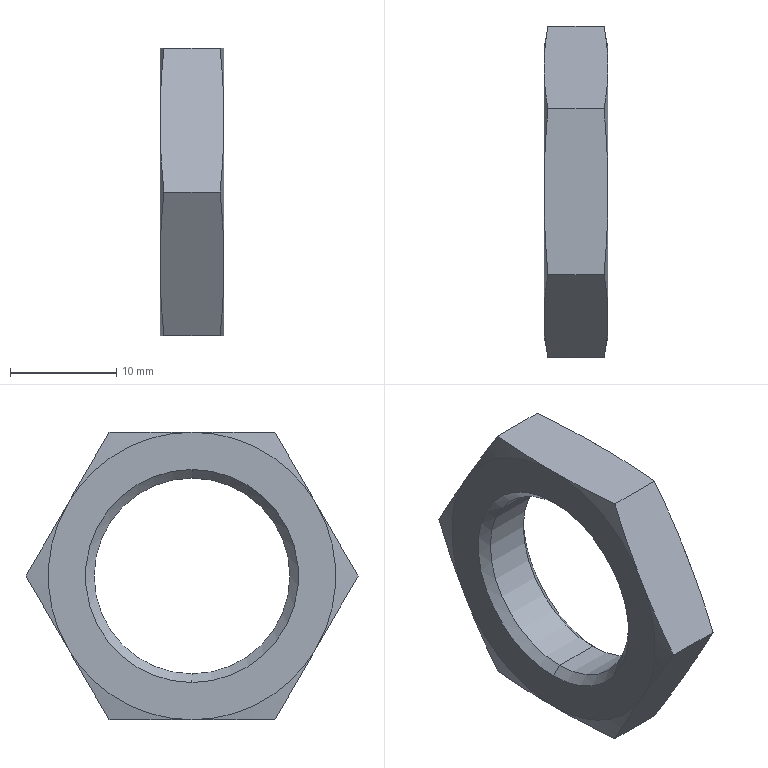Part | STEP file | 204596_DIN176_M20x1_5_7_24_HI | 1 solid | 26 faces | box 6 x 31.177 x 27 mm | volume 2144 mm3 | cone 16 | plane 8 | cylinder 2 | commonest cylinder face diameters 18.376 x2